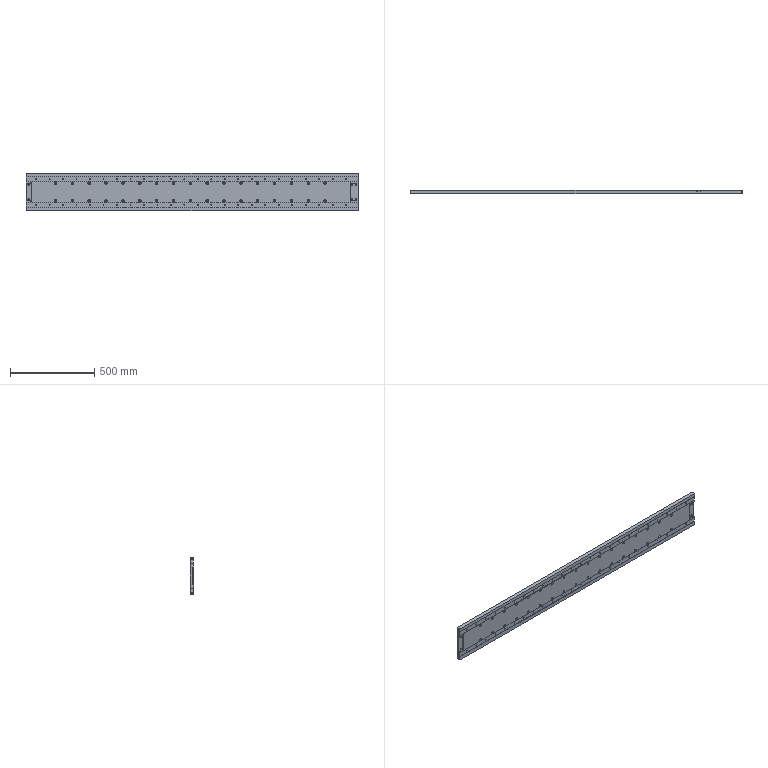Part | STEP file | 1 solid | 378 faces | box 1970 x 20 x 225 mm | volume 8481911 mm3 | cylinder 286 | plane 60 | cone 32 | commonest cylinder face diameters 5 x96 9 x68 15 x68 4.2 x24 8.5 x12 4 x6